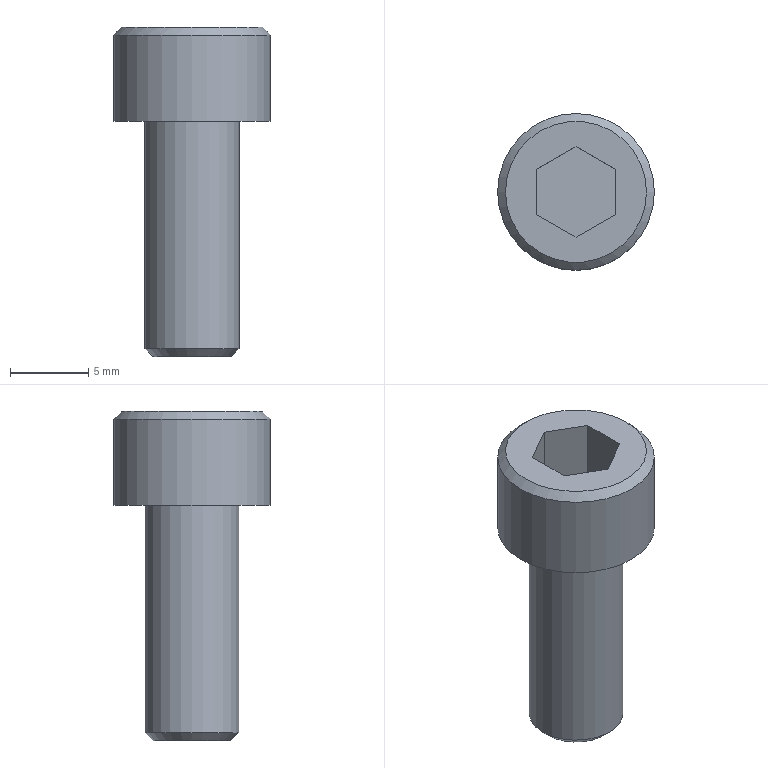Part | STEP file | gslz 2016.10.28-6_id686_x_t | 1 solid | 14 faces | box 10 x 10 x 21 mm | volume 802.73 mm3 | plane 10 | cylinder 2 | cone 2 | commonest cylinder face diameters 6 x1 10 x1
STEP:
#1=CARTESIAN_POINT('',(96.2,150.,44.));
#2=VERTEX_POINT('',#1);
#3=CARTESIAN_POINT('',(100.7,150.,44.));
#4=DIRECTION('',(0.,0.,-1.));
#5=DIRECTION('',(-1.,0.,0.));
#6=AXIS2_PLACEMENT_3D('',#3,#4,#5);
#7=CIRCLE('',#6,4.5);
#8=EDGE_CURVE('',#2,#2,#7,.T.);
#9=ORIENTED_EDGE('',*,*,#8,.F.);
#10=EDGE_LOOP('',(#9));
#11=FACE_BOUND('',#10,.T.);
#12=CARTESIAN_POINT('',(103.2,151.443,44.));
#13=VERTEX_POINT('',#12);
#14=CARTESIAN_POINT('',(103.2,148.556,44.));
#15=VERTEX_POINT('',#14);
#16=CARTESIAN_POINT('',(103.2,151.443,44.));
#17=DIRECTION('',(0.,-1.,0.));
#18=VECTOR('',#17,1.);
#19=LINE('',#16,#18);
#20=EDGE_CURVE('',#13,#15,#19,.T.);
#21=ORIENTED_EDGE('',*,*,#20,.T.);
#22=CARTESIAN_POINT('',(100.7,147.113,44.));
#23=VERTEX_POINT('',#22);
#24=CARTESIAN_POINT('',(103.2,148.556,44.));
#25=DIRECTION('',(-0.866,-0.5,0.));
#26=VECTOR('',#25,1.);
#27=LINE('',#24,#26);
#28=EDGE_CURVE('',#15,#23,#27,.T.);
#29=ORIENTED_EDGE('',*,*,#28,.T.);
#30=CARTESIAN_POINT('',(98.2,148.556,44.));
#31=VERTEX_POINT('',#30);
#32=CARTESIAN_POINT('',(100.7,147.113,44.));
#33=DIRECTION('',(-0.866,0.5,0.));
#34=VECTOR('',#33,1.);
#35=LINE('',#32,#34);
#36=EDGE_CURVE('',#23,#31,#35,.T.);
#37=ORIENTED_EDGE('',*,*,#36,.T.);
#38=CARTESIAN_POINT('',(98.2,151.443,44.));
#39=VERTEX_POINT('',#38);
#40=CARTESIAN_POINT('',(98.2,148.556,44.));
#41=DIRECTION('',(0.,1.,0.));
#42=VECTOR('',#41,1.);
#43=LINE('',#40,#42);
#44=EDGE_CURVE('',#31,#39,#43,.T.);
#45=ORIENTED_EDGE('',*,*,#44,.T.);
#46=CARTESIAN_POINT('',(100.7,152.886,44.));
#47=VERTEX_POINT('',#46);
#48=CARTESIAN_POINT('',(98.2,151.443,44.));
#49=DIRECTION('',(0.866,0.5,0.));
#50=VECTOR('',#49,1.);
#51=LINE('',#48,#50);
#52=EDGE_CURVE('',#39,#47,#51,.T.);
#53=ORIENTED_EDGE('',*,*,#52,.T.);
#54=CARTESIAN_POINT('',(100.7,152.886,44.));
#55=DIRECTION('',(0.866,-0.5,0.));
#56=VECTOR('',#55,1.);
#57=LINE('',#54,#56);
#58=EDGE_CURVE('',#47,#13,#57,.T.);
#59=ORIENTED_EDGE('',*,*,#58,.T.);
#60=EDGE_LOOP('',(#21,#29,#37,#45,#53,#59));
#61=FACE_BOUND('',#60,.T.);
#62=CARTESIAN_POINT('',(100.7,150.,44.));
#63=DIRECTION('',(0.,0.,1.));
#64=DIRECTION('',(1.,0.,0.));
#65=AXIS2_PLACEMENT_3D('',#62,#63,#64);
#66=PLANE('',#65);
#67=ADVANCED_FACE('',(#11,#61),#66,.T.);
#68=CARTESIAN_POINT('',(103.2,150.,23.));
#69=VERTEX_POINT('',#68);
#70=CARTESIAN_POINT('',(100.7,150.,23.));
#71=DIRECTION('',(0.,0.,1.));
#72=DIRECTION('',(1.,0.,0.));
#73=AXIS2_PLACEMENT_3D('',#70,#71,#72);
#74=CIRCLE('',#73,2.5);
#75=EDGE_CURVE('',#69,#69,#74,.T.);
#76=ORIENTED_EDGE('',*,*,#75,.F.);
#77=EDGE_LOOP('',(#76));
#78=FACE_OUTER_BOUND('',#77,.T.);
#79=CARTESIAN_POINT('',(100.7,150.,23.));
#80=DIRECTION('',(0.,0.,-1.));
#81=DIRECTION('',(-1.,0.,0.));
#82=AXIS2_PLACEMENT_3D('',#79,#80,#81);
#83=PLANE('',#82);
#84=ADVANCED_FACE('',(#78),#83,.T.);
#85=CARTESIAN_POINT('',(97.7,150.,23.5));
#86=VERTEX_POINT('',#85);
#87=CARTESIAN_POINT('',(100.7,150.,23.5));
#88=DIRECTION('',(0.,0.,-1.));
#89=DIRECTION('',(-1.,0.,0.));
#90=AXIS2_PLACEMENT_3D('',#87,#88,#89);
#91=CIRCLE('',#90,3.);
#92=EDGE_CURVE('',#86,#86,#91,.T.);
#93=ORIENTED_EDGE('',*,*,#92,.F.);
#94=EDGE_LOOP('',(#93));
#95=FACE_BOUND('',#94,.T.);
#96=CARTESIAN_POINT('',(103.7,150.,38.));
#97=VERTEX_POINT('',#96);
#98=CARTESIAN_POINT('',(100.7,150.,38.));
#99=DIRECTION('',(0.,0.,1.));
#100=DIRECTION('',(1.,0.,0.));
#101=AXIS2_PLACEMENT_3D('',#98,#99,#100);
#102=CIRCLE('',#101,3.);
#103=EDGE_CURVE('',#97,#97,#102,.T.);
#104=ORIENTED_EDGE('',*,*,#103,.F.);
#105=EDGE_LOOP('',(#104));
#106=FACE_BOUND('',#105,.T.);
#107=CARTESIAN_POINT('',(100.7,150.,32.));
#108=DIRECTION('',(0.,0.,-1.));
#109=DIRECTION('',(-1.,0.,0.));
#110=AXIS2_PLACEMENT_3D('',#107,#108,#109);
#111=CYLINDRICAL_SURFACE('',#110,3.);
#112=ADVANCED_FACE('',(#95,#106),#111,.T.);
#113=ORIENTED_EDGE('',*,*,#103,.T.);
#114=EDGE_LOOP('',(#113));
#115=FACE_BOUND('',#114,.T.);
#116=CARTESIAN_POINT('',(105.7,150.,38.));
#117=VERTEX_POINT('',#116);
#118=CARTESIAN_POINT('',(100.7,150.,38.));
#119=DIRECTION('',(0.,0.,1.));
#120=DIRECTION('',(1.,0.,0.));
#121=AXIS2_PLACEMENT_3D('',#118,#119,#120);
#122=CIRCLE('',#121,5.);
#123=EDGE_CURVE('',#117,#117,#122,.T.);
#124=ORIENTED_EDGE('',*,*,#123,.F.);
#125=EDGE_LOOP('',(#124));
#126=FACE_BOUND('',#125,.T.);
#127=CARTESIAN_POINT('',(100.7,150.,38.));
#128=DIRECTION('',(0.,0.,-1.));
#129=DIRECTION('',(-1.,0.,0.));
#130=AXIS2_PLACEMENT_3D('',#127,#128,#129);
#131=PLANE('',#130);
#132=ADVANCED_FACE('',(#115,#126),#131,.T.);
#133=CARTESIAN_POINT('',(95.7,150.,43.5));
#134=VERTEX_POINT('',#133);
#135=CARTESIAN_POINT('',(100.7,150.,43.5));
#136=DIRECTION('',(0.,0.,1.));
#137=DIRECTION('',(-1.,0.,0.));
#138=AXIS2_PLACEMENT_3D('',#135,#136,#137);
#139=CIRCLE('',#138,5.);
#140=EDGE_CURVE('',#134,#134,#139,.T.);
#141=ORIENTED_EDGE('',*,*,#140,.F.);
#142=EDGE_LOOP('',(#141));
#143=FACE_BOUND('',#142,.T.);
#144=ORIENTED_EDGE('',*,*,#123,.T.);
#145=EDGE_LOOP('',(#144));
#146=FACE_BOUND('',#145,.T.);
#147=CARTESIAN_POINT('',(100.7,150.,46.));
#148=DIRECTION('',(0.,0.,-1.));
#149=DIRECTION('',(-1.,0.,0.));
#150=AXIS2_PLACEMENT_3D('',#147,#148,#149);
#151=CYLINDRICAL_SURFACE('',#150,5.);
#152=ADVANCED_FACE('',(#143,#146),#151,.T.);
#153=ORIENTED_EDGE('',*,*,#92,.T.);
#154=EDGE_LOOP('',(#153));
#155=FACE_BOUND('',#154,.T.);
#156=ORIENTED_EDGE('',*,*,#75,.T.);
#157=EDGE_LOOP('',(#156));
#158=FACE_BOUND('',#157,.T.);
#159=CARTESIAN_POINT('',(100.7,150.,23.));
#160=DIRECTION('',(0.,0.,1.));
#161=DIRECTION('',(-1.,0.,0.));
#162=AXIS2_PLACEMENT_3D('',#159,#160,#161);
#163=CONICAL_SURFACE('',#162,2.5,45.);
#164=ADVANCED_FACE('',(#155,#158),#163,.T.);
#165=ORIENTED_EDGE('',*,*,#20,.F.);
#166=CARTESIAN_POINT('',(103.2,151.443,40.));
#167=VERTEX_POINT('',#166);
#168=CARTESIAN_POINT('',(103.2,151.443,40.));
#169=DIRECTION('',(0.,0.,-1.));
#170=VECTOR('',#169,1.);
#171=LINE('',#168,#170);
#172=EDGE_CURVE('',#13,#167,#171,.T.);
#173=ORIENTED_EDGE('',*,*,#172,.T.);
#174=CARTESIAN_POINT('',(103.2,148.556,40.));
#175=VERTEX_POINT('',#174);
#176=CARTESIAN_POINT('',(103.2,151.443,40.));
#177=DIRECTION('',(0.,1.,0.));
#178=VECTOR('',#177,1.);
#179=LINE('',#176,#178);
#180=EDGE_CURVE('',#175,#167,#179,.T.);
#181=ORIENTED_EDGE('',*,*,#180,.F.);
#182=CARTESIAN_POINT('',(103.2,148.556,40.));
#183=DIRECTION('',(0.,0.,-1.));
#184=VECTOR('',#183,1.);
#185=LINE('',#182,#184);
#186=EDGE_CURVE('',#15,#175,#185,.T.);
#187=ORIENTED_EDGE('',*,*,#186,.F.);
#188=EDGE_LOOP('',(#165,#173,#181,#187));
#189=FACE_OUTER_BOUND('',#188,.T.);
#190=CARTESIAN_POINT('',(103.2,151.443,40.));
#191=DIRECTION('',(1.,0.,0.));
#192=DIRECTION('',(0.,1.,0.));
#193=AXIS2_PLACEMENT_3D('',#190,#191,#192);
#194=PLANE('',#193);
#195=ADVANCED_FACE('',(#189),#194,.F.);
#196=ORIENTED_EDGE('',*,*,#28,.F.);
#197=ORIENTED_EDGE('',*,*,#186,.T.);
#198=CARTESIAN_POINT('',(100.7,147.113,40.));
#199=VERTEX_POINT('',#198);
#200=CARTESIAN_POINT('',(103.2,148.556,40.));
#201=DIRECTION('',(0.866,0.5,0.));
#202=VECTOR('',#201,1.);
#203=LINE('',#200,#202);
#204=EDGE_CURVE('',#199,#175,#203,.T.);
#205=ORIENTED_EDGE('',*,*,#204,.F.);
#206=CARTESIAN_POINT('',(100.7,147.113,40.));
#207=DIRECTION('',(0.,0.,-1.));
#208=VECTOR('',#207,1.);
#209=LINE('',#206,#208);
#210=EDGE_CURVE('',#23,#199,#209,.T.);
#211=ORIENTED_EDGE('',*,*,#210,.F.);
#212=EDGE_LOOP('',(#196,#197,#205,#211));
#213=FACE_OUTER_BOUND('',#212,.T.);
#214=CARTESIAN_POINT('',(103.2,148.556,40.));
#215=DIRECTION('',(0.5,-0.866,0.));
#216=DIRECTION('',(0.866,0.5,0.));
#217=AXIS2_PLACEMENT_3D('',#214,#215,#216);
#218=PLANE('',#217);
#219=ADVANCED_FACE('',(#213),#218,.F.);
#220=ORIENTED_EDGE('',*,*,#36,.F.);
#221=ORIENTED_EDGE('',*,*,#210,.T.);
#222=CARTESIAN_POINT('',(98.2,148.556,40.));
#223=VERTEX_POINT('',#222);
#224=CARTESIAN_POINT('',(100.7,147.113,40.));
#225=DIRECTION('',(0.866,-0.5,0.));
#226=VECTOR('',#225,1.);
#227=LINE('',#224,#226);
#228=EDGE_CURVE('',#223,#199,#227,.T.);
#229=ORIENTED_EDGE('',*,*,#228,.F.);
#230=CARTESIAN_POINT('',(98.2,148.556,40.));
#231=DIRECTION('',(0.,0.,-1.));
#232=VECTOR('',#231,1.);
#233=LINE('',#230,#232);
#234=EDGE_CURVE('',#31,#223,#233,.T.);
#235=ORIENTED_EDGE('',*,*,#234,.F.);
#236=EDGE_LOOP('',(#220,#221,#229,#235));
#237=FACE_OUTER_BOUND('',#236,.T.);
#238=CARTESIAN_POINT('',(100.7,147.113,40.));
#239=DIRECTION('',(-0.5,-0.866,0.));
#240=DIRECTION('',(0.866,-0.5,0.));
#241=AXIS2_PLACEMENT_3D('',#238,#239,#240);
#242=PLANE('',#241);
#243=ADVANCED_FACE('',(#237),#242,.F.);
#244=ORIENTED_EDGE('',*,*,#44,.F.);
#245=ORIENTED_EDGE('',*,*,#234,.T.);
#246=CARTESIAN_POINT('',(98.2,151.443,40.));
#247=VERTEX_POINT('',#246);
#248=CARTESIAN_POINT('',(98.2,148.556,40.));
#249=DIRECTION('',(0.,-1.,0.));
#250=VECTOR('',#249,1.);
#251=LINE('',#248,#250);
#252=EDGE_CURVE('',#247,#223,#251,.T.);
#253=ORIENTED_EDGE('',*,*,#252,.F.);
#254=CARTESIAN_POINT('',(98.2,151.443,40.));
#255=DIRECTION('',(0.,0.,-1.));
#256=VECTOR('',#255,1.);
#257=LINE('',#254,#256);
#258=EDGE_CURVE('',#39,#247,#257,.T.);
#259=ORIENTED_EDGE('',*,*,#258,.F.);
#260=EDGE_LOOP('',(#244,#245,#253,#259));
#261=FACE_OUTER_BOUND('',#260,.T.);
#262=CARTESIAN_POINT('',(98.2,148.556,40.));
#263=DIRECTION('',(-1.,0.,0.));
#264=DIRECTION('',(0.,0.,1.));
#265=AXIS2_PLACEMENT_3D('',#262,#263,#264);
#266=PLANE('',#265);
#267=ADVANCED_FACE('',(#261),#266,.F.);
#268=ORIENTED_EDGE('',*,*,#52,.F.);
#269=ORIENTED_EDGE('',*,*,#258,.T.);
#270=CARTESIAN_POINT('',(100.7,152.886,40.));
#271=VERTEX_POINT('',#270);
#272=CARTESIAN_POINT('',(98.2,151.443,40.));
#273=DIRECTION('',(-0.866,-0.5,0.));
#274=VECTOR('',#273,1.);
#275=LINE('',#272,#274);
#276=EDGE_CURVE('',#271,#247,#275,.T.);
#277=ORIENTED_EDGE('',*,*,#276,.F.);
#278=CARTESIAN_POINT('',(100.7,152.886,40.));
#279=DIRECTION('',(0.,0.,-1.));
#280=VECTOR('',#279,1.);
#281=LINE('',#278,#280);
#282=EDGE_CURVE('',#47,#271,#281,.T.);
#283=ORIENTED_EDGE('',*,*,#282,.F.);
#284=EDGE_LOOP('',(#268,#269,#277,#283));
#285=FACE_OUTER_BOUND('',#284,.T.);
#286=CARTESIAN_POINT('',(98.2,151.443,40.));
#287=DIRECTION('',(-0.5,0.866,0.));
#288=DIRECTION('',(-0.866,-0.5,0.));
#289=AXIS2_PLACEMENT_3D('',#286,#287,#288);
#290=PLANE('',#289);
#291=ADVANCED_FACE('',(#285),#290,.F.);
#292=ORIENTED_EDGE('',*,*,#58,.F.);
#293=ORIENTED_EDGE('',*,*,#282,.T.);
#294=CARTESIAN_POINT('',(100.7,152.886,40.));
#295=DIRECTION('',(-0.866,0.5,0.));
#296=VECTOR('',#295,1.);
#297=LINE('',#294,#296);
#298=EDGE_CURVE('',#167,#271,#297,.T.);
#299=ORIENTED_EDGE('',*,*,#298,.F.);
#300=ORIENTED_EDGE('',*,*,#172,.F.);
#301=EDGE_LOOP('',(#292,#293,#299,#300));
#302=FACE_OUTER_BOUND('',#301,.T.);
#303=CARTESIAN_POINT('',(100.7,152.886,40.));
#304=DIRECTION('',(0.5,0.866,0.));
#305=DIRECTION('',(-0.866,0.5,0.));
#306=AXIS2_PLACEMENT_3D('',#303,#304,#305);
#307=PLANE('',#306);
#308=ADVANCED_FACE('',(#302),#307,.F.);
#309=ORIENTED_EDGE('',*,*,#180,.T.);
#310=ORIENTED_EDGE('',*,*,#298,.T.);
#311=ORIENTED_EDGE('',*,*,#276,.T.);
#312=ORIENTED_EDGE('',*,*,#252,.T.);
#313=ORIENTED_EDGE('',*,*,#228,.T.);
#314=ORIENTED_EDGE('',*,*,#204,.T.);
#315=EDGE_LOOP('',(#309,#310,#311,#312,#313,#314));
#316=FACE_OUTER_BOUND('',#315,.T.);
#317=CARTESIAN_POINT('',(103.2,148.556,40.));
#318=DIRECTION('',(0.,0.,1.));
#319=DIRECTION('',(1.,0.,0.));
#320=AXIS2_PLACEMENT_3D('',#317,#318,#319);
#321=PLANE('',#320);
#322=ADVANCED_FACE('',(#316),#321,.T.);
#323=ORIENTED_EDGE('',*,*,#8,.T.);
#324=EDGE_LOOP('',(#323));
#325=FACE_BOUND('',#324,.T.);
#326=ORIENTED_EDGE('',*,*,#140,.T.);
#327=EDGE_LOOP('',(#326));
#328=FACE_BOUND('',#327,.T.);
#329=CARTESIAN_POINT('',(100.7,150.,43.5));
#330=DIRECTION('',(0.,0.,-1.));
#331=DIRECTION('',(-1.,0.,0.));
#332=AXIS2_PLACEMENT_3D('',#329,#330,#331);
#333=CONICAL_SURFACE('',#332,5.,45.);
#334=ADVANCED_FACE('',(#325,#328),#333,.T.);
#335=CLOSED_SHELL('',(#67,#84,#112,#132,#152,#164,#195,#219,#243,#267,#291,#308,#322,#334));
#336=MANIFOLD_SOLID_BREP('',#335);
#337=(LENGTH_UNIT()NAMED_UNIT(*)SI_UNIT(.MILLI.,.METRE.));
#338=UNCERTAINTY_MEASURE_WITH_UNIT(LENGTH_MEASURE(0.00002),#337,'','');
#339=(NAMED_UNIT(*)PLANE_ANGLE_UNIT()SI_UNIT($,.RADIAN.));
#340=PLANE_ANGLE_MEASURE_WITH_UNIT(PLANE_ANGLE_MEASURE(0.01745),#339);
#341=DIMENSIONAL_EXPONENTS(0.,0.,0.,0.,0.,0.,0.);
#342=(CONVERSION_BASED_UNIT('DEGREE',#340)NAMED_UNIT(#341)PLANE_ANGLE_UNIT());
#343=(NAMED_UNIT(*)SI_UNIT($,.STERADIAN.)SOLID_ANGLE_UNIT());
#344=(GEOMETRIC_REPRESENTATION_CONTEXT(3)GLOBAL_UNCERTAINTY_ASSIGNED_CONTEXT((#338))GLOBAL_UNIT_ASSIGNED_CONTEXT((#337,#342,#343))REPRESENTATION_CONTEXT('',''));
#345=ADVANCED_BREP_SHAPE_REPRESENTATION('',(#336),#344);